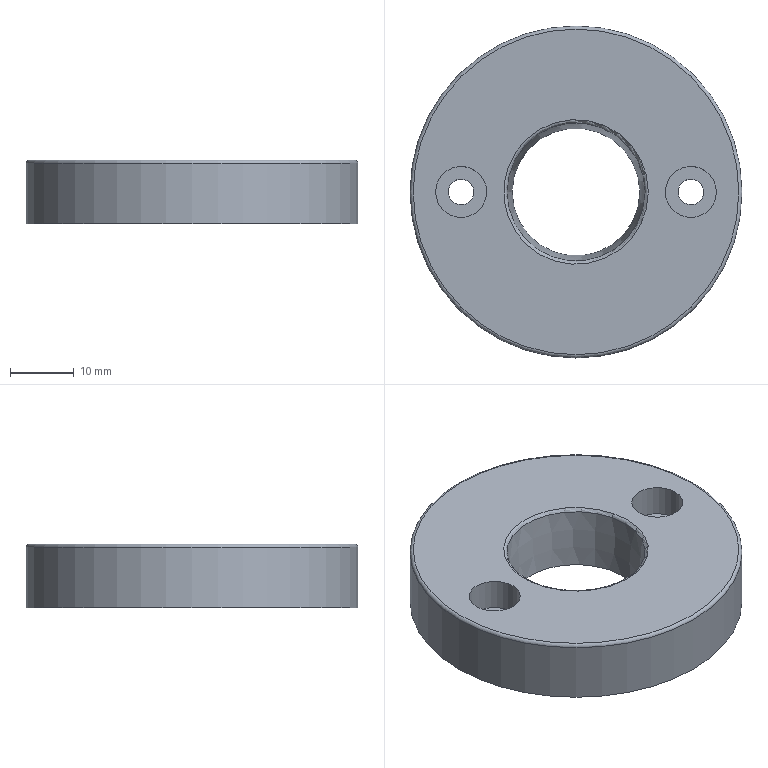Part | STEP file | DISCO_BASE_ALIMENTADOR_PINO | 1 solid | 12 faces | box 52 x 52 x 10 mm | volume 17173 mm3 | cylinder 5 | plane 4 | torus 2 | cone 1 | commonest cylinder face diameters 4 x2 8 x2 52 x1
STEP:
#1=CARTESIAN_POINT('',(0.,0.,0.));
#2=DIRECTION('',(0.,0.,1.));
#3=DIRECTION('',(1.,0.,0.));
#4=AXIS2_PLACEMENT_3D('',#1,#2,#3);
#5=CARTESIAN_POINT('',(-21.51,1.918,5.));
#6=VERTEX_POINT('',#5);
#7=CARTESIAN_POINT('',(-18.,0.,5.));
#8=DIRECTION('',(0.,0.,-1.));
#9=DIRECTION('',(1.,0.,0.));
#10=AXIS2_PLACEMENT_3D('',#7,#8,#9);
#11=CIRCLE('',#10,4.);
#12=CARTESIAN_POINT('',(-16.,0.,5.));
#13=DIRECTION('',(0.,0.,-1.));
#14=DIRECTION('',(-1.,0.,0.));
#15=AXIS2_PLACEMENT_3D('',#12,#13,#14);
#16=PLANE('',#15);
#17=CARTESIAN_POINT('',(2.,0.));
#18=DIRECTION('',(-1.,0.));
#19=AXIS2_PLACEMENT_2D('',#17,#18);
#20=CIRCLE('',#19,4.);
#21=(GEOMETRIC_REPRESENTATION_CONTEXT(2)PARAMETRIC_REPRESENTATION_CONTEXT()REPRESENTATION_CONTEXT('',''));
#22=DEFINITIONAL_REPRESENTATION('',(#20),#21);
#23=PCURVE('',#16,#22);
#24=CARTESIAN_POINT('',(-18.,0.,9.9));
#25=DIRECTION('',(0.,0.,-1.));
#26=DIRECTION('',(0.8776,-0.4794,0.));
#27=AXIS2_PLACEMENT_3D('',#24,#25,#26);
#28=CYLINDRICAL_SURFACE('',#27,4.);
#29=CARTESIAN_POINT('',(-0.5,4.9));
#30=DIRECTION('',(1.,0.));
#31=VECTOR('',#30,1.);
#32=LINE('',#29,#31);
#33=(GEOMETRIC_REPRESENTATION_CONTEXT(2)PARAMETRIC_REPRESENTATION_CONTEXT()REPRESENTATION_CONTEXT('',''));
#34=DEFINITIONAL_REPRESENTATION('',(#32),#33);
#35=PCURVE('',#28,#34);
#36=SURFACE_CURVE('',#11,(#23,#35),.PCURVE_S1.);
#37=EDGE_CURVE('',#6,#6,#36,.T.);
#38=ORIENTED_EDGE('',*,*,#37,.F.);
#39=EDGE_LOOP('',(#38));
#40=FACE_BOUND('',#39,.T.);
#41=CARTESIAN_POINT('',(-16.245,-0.9589,5.));
#42=VERTEX_POINT('',#41);
#43=CARTESIAN_POINT('',(-18.,0.,5.));
#44=DIRECTION('',(0.,0.,-1.));
#45=DIRECTION('',(1.,0.,0.));
#46=AXIS2_PLACEMENT_3D('',#43,#44,#45);
#47=CIRCLE('',#46,2.);
#48=CARTESIAN_POINT('',(2.,0.));
#49=DIRECTION('',(-1.,0.));
#50=AXIS2_PLACEMENT_2D('',#48,#49);
#51=CIRCLE('',#50,2.);
#52=(GEOMETRIC_REPRESENTATION_CONTEXT(2)PARAMETRIC_REPRESENTATION_CONTEXT()REPRESENTATION_CONTEXT('',''));
#53=DEFINITIONAL_REPRESENTATION('',(#51),#52);
#54=PCURVE('',#16,#53);
#55=CARTESIAN_POINT('',(-18.,0.,9.9));
#56=DIRECTION('',(0.,0.,-1.));
#57=DIRECTION('',(0.8776,-0.4794,0.));
#58=AXIS2_PLACEMENT_3D('',#55,#56,#57);
#59=CYLINDRICAL_SURFACE('',#58,2.);
#60=CARTESIAN_POINT('',(-0.5,4.9));
#61=DIRECTION('',(1.,0.));
#62=VECTOR('',#61,1.);
#63=LINE('',#60,#62);
#64=(GEOMETRIC_REPRESENTATION_CONTEXT(2)PARAMETRIC_REPRESENTATION_CONTEXT()REPRESENTATION_CONTEXT('',''));
#65=DEFINITIONAL_REPRESENTATION('',(#63),#64);
#66=PCURVE('',#59,#65);
#67=SURFACE_CURVE('',#47,(#54,#66),.PCURVE_S1.);
#68=EDGE_CURVE('',#42,#42,#67,.T.);
#69=ORIENTED_EDGE('',*,*,#68,.T.);
#70=EDGE_LOOP('',(#69));
#71=FACE_BOUND('',#70,.T.);
#72=ADVANCED_FACE('',(#40,#71),#16,.F.);
#73=CARTESIAN_POINT('',(-16.245,-0.9589,0.));
#74=VERTEX_POINT('',#73);
#75=CARTESIAN_POINT('',(-18.,0.,0.));
#76=DIRECTION('',(0.,0.,-1.));
#77=DIRECTION('',(1.,0.,0.));
#78=AXIS2_PLACEMENT_3D('',#75,#76,#77);
#79=CIRCLE('',#78,2.);
#80=CARTESIAN_POINT('',(-0.5,9.9));
#81=DIRECTION('',(1.,0.));
#82=VECTOR('',#81,1.);
#83=LINE('',#80,#82);
#84=(GEOMETRIC_REPRESENTATION_CONTEXT(2)PARAMETRIC_REPRESENTATION_CONTEXT()REPRESENTATION_CONTEXT('',''));
#85=DEFINITIONAL_REPRESENTATION('',(#83),#84);
#86=PCURVE('',#59,#85);
#87=CARTESIAN_POINT('',(0.,0.,0.));
#88=DIRECTION('',(0.,0.,1.));
#89=DIRECTION('',(1.,0.,0.));
#90=AXIS2_PLACEMENT_3D('',#87,#88,#89);
#91=PLANE('',#90);
#92=CARTESIAN_POINT('',(-16.,0.));
#93=CARTESIAN_POINT('',(-16.,-3.464));
#94=CARTESIAN_POINT('',(-19.,-1.732));
#95=CARTESIAN_POINT('',(-22.,0.));
#96=CARTESIAN_POINT('',(-19.,1.732));
#97=CARTESIAN_POINT('',(-16.,3.464));
#98=CARTESIAN_POINT('',(-16.,0.));
#99=(BOUNDED_CURVE()B_SPLINE_CURVE(2,(#92,#93,#94,#95,#96,#97,#98),.UNSPECIFIED.,.T.,.F.)B_SPLINE_CURVE_WITH_KNOTS((1,2,2,2,2,1),(-2.094,0.,2.094,4.189,6.283,8.378),.UNSPECIFIED.)CURVE()GEOMETRIC_REPRESENTATION_ITEM()RATIONAL_B_SPLINE_CURVE((1.,0.5,1.,0.5,1.,0.5,1.))REPRESENTATION_ITEM(''));
#100=(GEOMETRIC_REPRESENTATION_CONTEXT(2)PARAMETRIC_REPRESENTATION_CONTEXT()REPRESENTATION_CONTEXT('',''));
#101=DEFINITIONAL_REPRESENTATION('',(#99),#100);
#102=PCURVE('',#91,#101);
#103=SURFACE_CURVE('',#79,(#86,#102),.PCURVE_S1.);
#104=EDGE_CURVE('',#74,#74,#103,.T.);
#105=ORIENTED_EDGE('',*,*,#104,.F.);
#106=CARTESIAN_POINT('',(-16.245,-0.9589,5.));
#107=CARTESIAN_POINT('',(-16.245,-0.9589,0.));
#108=B_SPLINE_CURVE_WITH_KNOTS('',1,(#106,#107),.UNSPECIFIED.,.F.,.F.,(2,2),(4.9,9.9),.PIECEWISE_BEZIER_KNOTS.);
#109=CARTESIAN_POINT('',(0.,0.));
#110=DIRECTION('',(0.,1.));
#111=VECTOR('',#110,1.);
#112=LINE('',#109,#111);
#113=(GEOMETRIC_REPRESENTATION_CONTEXT(2)PARAMETRIC_REPRESENTATION_CONTEXT()REPRESENTATION_CONTEXT('',''));
#114=DEFINITIONAL_REPRESENTATION('',(#112),#113);
#115=PCURVE('',#59,#114);
#116=CARTESIAN_POINT('',(6.283,0.));
#117=DIRECTION('',(0.,1.));
#118=VECTOR('',#117,1.);
#119=LINE('',#116,#118);
#120=(GEOMETRIC_REPRESENTATION_CONTEXT(2)PARAMETRIC_REPRESENTATION_CONTEXT()REPRESENTATION_CONTEXT('',''));
#121=DEFINITIONAL_REPRESENTATION('',(#119),#120);
#122=PCURVE('',#59,#121);
#123=SEAM_CURVE('',#108,(#115,#122),.PCURVE_S1.);
#124=EDGE_CURVE('',#42,#74,#123,.T.);
#125=ORIENTED_EDGE('',*,*,#124,.F.);
#126=ORIENTED_EDGE('',*,*,#68,.T.);
#127=ORIENTED_EDGE('',*,*,#124,.T.);
#128=EDGE_LOOP('',(#105,#125,#126,#127));
#129=FACE_BOUND('',#128,.F.);
#130=ADVANCED_FACE('',(#129),#59,.F.);
#131=CARTESIAN_POINT('',(-21.51,1.918,10.));
#132=VERTEX_POINT('',#131);
#133=CARTESIAN_POINT('',(-18.,0.,10.));
#134=DIRECTION('',(0.,0.,-1.));
#135=DIRECTION('',(1.,0.,0.));
#136=AXIS2_PLACEMENT_3D('',#133,#134,#135);
#137=CIRCLE('',#136,4.);
#138=CARTESIAN_POINT('',(-0.5,-0.1));
#139=DIRECTION('',(1.,0.));
#140=VECTOR('',#139,1.);
#141=LINE('',#138,#140);
#142=(GEOMETRIC_REPRESENTATION_CONTEXT(2)PARAMETRIC_REPRESENTATION_CONTEXT()REPRESENTATION_CONTEXT('',''));
#143=DEFINITIONAL_REPRESENTATION('',(#141),#142);
#144=PCURVE('',#28,#143);
#145=CARTESIAN_POINT('',(0.,0.,10.));
#146=DIRECTION('',(0.,0.,1.));
#147=DIRECTION('',(1.,0.,0.));
#148=AXIS2_PLACEMENT_3D('',#145,#146,#147);
#149=PLANE('',#148);
#150=CARTESIAN_POINT('',(-14.,0.));
#151=CARTESIAN_POINT('',(-14.,-6.928));
#152=CARTESIAN_POINT('',(-20.,-3.464));
#153=CARTESIAN_POINT('',(-26.,0.));
#154=CARTESIAN_POINT('',(-20.,3.464));
#155=CARTESIAN_POINT('',(-14.,6.928));
#156=CARTESIAN_POINT('',(-14.,0.));
#157=(BOUNDED_CURVE()B_SPLINE_CURVE(2,(#150,#151,#152,#153,#154,#155,#156),.UNSPECIFIED.,.T.,.F.)B_SPLINE_CURVE_WITH_KNOTS((1,2,2,2,2,1),(-2.094,0.,2.094,4.189,6.283,8.378),.UNSPECIFIED.)CURVE()GEOMETRIC_REPRESENTATION_ITEM()RATIONAL_B_SPLINE_CURVE((1.,0.5,1.,0.5,1.,0.5,1.))REPRESENTATION_ITEM(''));
#158=(GEOMETRIC_REPRESENTATION_CONTEXT(2)PARAMETRIC_REPRESENTATION_CONTEXT()REPRESENTATION_CONTEXT('',''));
#159=DEFINITIONAL_REPRESENTATION('',(#157),#158);
#160=PCURVE('',#149,#159);
#161=SURFACE_CURVE('',#137,(#144,#160),.PCURVE_S1.);
#162=EDGE_CURVE('',#132,#132,#161,.T.);
#163=ORIENTED_EDGE('',*,*,#162,.T.);
#164=CARTESIAN_POINT('',(-21.51,1.918,10.));
#165=CARTESIAN_POINT('',(-21.51,1.918,5.));
#166=B_SPLINE_CURVE_WITH_KNOTS('',1,(#164,#165),.UNSPECIFIED.,.F.,.F.,(2,2),(-0.1,4.9),.PIECEWISE_BEZIER_KNOTS.);
#167=CARTESIAN_POINT('',(9.425,0.));
#168=DIRECTION('',(0.,1.));
#169=VECTOR('',#168,1.);
#170=LINE('',#167,#169);
#171=(GEOMETRIC_REPRESENTATION_CONTEXT(2)PARAMETRIC_REPRESENTATION_CONTEXT()REPRESENTATION_CONTEXT('',''));
#172=DEFINITIONAL_REPRESENTATION('',(#170),#171);
#173=PCURVE('',#28,#172);
#174=CARTESIAN_POINT('',(3.142,0.));
#175=DIRECTION('',(0.,1.));
#176=VECTOR('',#175,1.);
#177=LINE('',#174,#176);
#178=(GEOMETRIC_REPRESENTATION_CONTEXT(2)PARAMETRIC_REPRESENTATION_CONTEXT()REPRESENTATION_CONTEXT('',''));
#179=DEFINITIONAL_REPRESENTATION('',(#177),#178);
#180=PCURVE('',#28,#179);
#181=SEAM_CURVE('',#166,(#173,#180),.PCURVE_S1.);
#182=EDGE_CURVE('',#132,#6,#181,.T.);
#183=ORIENTED_EDGE('',*,*,#182,.T.);
#184=ORIENTED_EDGE('',*,*,#37,.F.);
#185=ORIENTED_EDGE('',*,*,#182,.F.);
#186=EDGE_LOOP('',(#163,#183,#184,#185));
#187=FACE_BOUND('',#186,.F.);
#188=ADVANCED_FACE('',(#187),#28,.F.);
#189=CARTESIAN_POINT('',(-26.,0.,0.));
#190=VERTEX_POINT('',#189);
#191=CARTESIAN_POINT('',(0.,0.,0.));
#192=DIRECTION('',(0.,0.,1.));
#193=DIRECTION('',(1.,0.,0.));
#194=AXIS2_PLACEMENT_3D('',#191,#192,#193);
#195=CIRCLE('',#194,26.);
#196=CARTESIAN_POINT('',(0.,0.));
#197=DIRECTION('',(1.,0.));
#198=AXIS2_PLACEMENT_2D('',#196,#197);
#199=CIRCLE('',#198,26.);
#200=(GEOMETRIC_REPRESENTATION_CONTEXT(2)PARAMETRIC_REPRESENTATION_CONTEXT()REPRESENTATION_CONTEXT('',''));
#201=DEFINITIONAL_REPRESENTATION('',(#199),#200);
#202=PCURVE('',#91,#201);
#203=CARTESIAN_POINT('',(0.,0.,5.));
#204=DIRECTION('',(0.,0.,1.));
#205=DIRECTION('',(1.,0.,0.));
#206=AXIS2_PLACEMENT_3D('',#203,#204,#205);
#207=CYLINDRICAL_SURFACE('',#206,26.);
#208=CARTESIAN_POINT('',(0.,-5.));
#209=DIRECTION('',(1.,0.));
#210=VECTOR('',#209,1.);
#211=LINE('',#208,#210);
#212=(GEOMETRIC_REPRESENTATION_CONTEXT(2)PARAMETRIC_REPRESENTATION_CONTEXT()REPRESENTATION_CONTEXT('',''));
#213=DEFINITIONAL_REPRESENTATION('',(#211),#212);
#214=PCURVE('',#207,#213);
#215=SURFACE_CURVE('',#195,(#202,#214),.PCURVE_S1.);
#216=EDGE_CURVE('',#190,#190,#215,.T.);
#217=ORIENTED_EDGE('',*,*,#216,.F.);
#218=EDGE_LOOP('',(#217));
#219=FACE_BOUND('',#218,.T.);
#220=CARTESIAN_POINT('',(16.245,0.9589,0.));
#221=VERTEX_POINT('',#220);
#222=CARTESIAN_POINT('',(18.,0.,0.));
#223=DIRECTION('',(0.,0.,1.));
#224=DIRECTION('',(1.,0.,0.));
#225=AXIS2_PLACEMENT_3D('',#222,#223,#224);
#226=CIRCLE('',#225,2.);
#227=CARTESIAN_POINT('',(18.,0.));
#228=DIRECTION('',(1.,0.));
#229=AXIS2_PLACEMENT_2D('',#227,#228);
#230=CIRCLE('',#229,2.);
#231=(GEOMETRIC_REPRESENTATION_CONTEXT(2)PARAMETRIC_REPRESENTATION_CONTEXT()REPRESENTATION_CONTEXT('',''));
#232=DEFINITIONAL_REPRESENTATION('',(#230),#231);
#233=PCURVE('',#91,#232);
#234=CARTESIAN_POINT('',(18.,0.,9.9));
#235=DIRECTION('',(0.,0.,-1.));
#236=DIRECTION('',(-0.8776,0.4794,0.));
#237=AXIS2_PLACEMENT_3D('',#234,#235,#236);
#238=CYLINDRICAL_SURFACE('',#237,2.);
#239=CARTESIAN_POINT('',(8.925,9.9));
#240=DIRECTION('',(-1.,0.));
#241=VECTOR('',#240,1.);
#242=LINE('',#239,#241);
#243=(GEOMETRIC_REPRESENTATION_CONTEXT(2)PARAMETRIC_REPRESENTATION_CONTEXT()REPRESENTATION_CONTEXT('',''));
#244=DEFINITIONAL_REPRESENTATION('',(#242),#243);
#245=PCURVE('',#238,#244);
#246=SURFACE_CURVE('',#226,(#233,#245),.PCURVE_S1.);
#247=EDGE_CURVE('',#221,#221,#246,.T.);
#248=ORIENTED_EDGE('',*,*,#247,.T.);
#249=EDGE_LOOP('',(#248));
#250=FACE_BOUND('',#249,.T.);
#251=ORIENTED_EDGE('',*,*,#104,.F.);
#252=EDGE_LOOP('',(#251));
#253=FACE_BOUND('',#252,.T.);
#254=CARTESIAN_POINT('',(-10.,0.,0.));
#255=VERTEX_POINT('',#254);
#256=CARTESIAN_POINT('',(0.,0.,0.));
#257=DIRECTION('',(0.,0.,1.));
#258=DIRECTION('',(1.,0.,0.));
#259=AXIS2_PLACEMENT_3D('',#256,#257,#258);
#260=CIRCLE('',#259,10.);
#261=CARTESIAN_POINT('',(0.,0.));
#262=DIRECTION('',(1.,0.));
#263=AXIS2_PLACEMENT_2D('',#261,#262);
#264=CIRCLE('',#263,10.);
#265=(GEOMETRIC_REPRESENTATION_CONTEXT(2)PARAMETRIC_REPRESENTATION_CONTEXT()REPRESENTATION_CONTEXT('',''));
#266=DEFINITIONAL_REPRESENTATION('',(#264),#265);
#267=PCURVE('',#91,#266);
#268=CARTESIAN_POINT('',(0.,0.,0.));
#269=DIRECTION('',(0.,0.,1.));
#270=DIRECTION('',(-1.,0.,0.));
#271=AXIS2_PLACEMENT_3D('',#268,#269,#270);
#272=CONICAL_SURFACE('',#271,10.,0.08727);
#273=CARTESIAN_POINT('',(-3.142,0.));
#274=DIRECTION('',(1.,0.));
#275=VECTOR('',#274,1.);
#276=LINE('',#273,#275);
#277=(GEOMETRIC_REPRESENTATION_CONTEXT(2)PARAMETRIC_REPRESENTATION_CONTEXT()REPRESENTATION_CONTEXT('',''));
#278=DEFINITIONAL_REPRESENTATION('',(#276),#277);
#279=PCURVE('',#272,#278);
#280=SURFACE_CURVE('',#260,(#267,#279),.PCURVE_S1.);
#281=EDGE_CURVE('',#255,#255,#280,.T.);
#282=ORIENTED_EDGE('',*,*,#281,.T.);
#283=EDGE_LOOP('',(#282));
#284=FACE_BOUND('',#283,.T.);
#285=ADVANCED_FACE('',(#219,#250,#253,#284),#91,.F.);
#286=CARTESIAN_POINT('',(14.49,1.918,5.));
#287=VERTEX_POINT('',#286);
#288=CARTESIAN_POINT('',(18.,0.,5.));
#289=DIRECTION('',(0.,0.,-1.));
#290=DIRECTION('',(1.,0.,0.));
#291=AXIS2_PLACEMENT_3D('',#288,#289,#290);
#292=CIRCLE('',#291,4.);
#293=CARTESIAN_POINT('',(-16.,0.,5.));
#294=DIRECTION('',(0.,0.,-1.));
#295=DIRECTION('',(-1.,0.,0.));
#296=AXIS2_PLACEMENT_3D('',#293,#294,#295);
#297=PLANE('',#296);
#298=CARTESIAN_POINT('',(-34.,0.));
#299=DIRECTION('',(-1.,0.));
#300=AXIS2_PLACEMENT_2D('',#298,#299);
#301=CIRCLE('',#300,4.);
#302=(GEOMETRIC_REPRESENTATION_CONTEXT(2)PARAMETRIC_REPRESENTATION_CONTEXT()REPRESENTATION_CONTEXT('',''));
#303=DEFINITIONAL_REPRESENTATION('',(#301),#302);
#304=PCURVE('',#297,#303);
#305=CARTESIAN_POINT('',(18.,0.,9.9));
#306=DIRECTION('',(0.,0.,-1.));
#307=DIRECTION('',(-0.8776,0.4794,0.));
#308=AXIS2_PLACEMENT_3D('',#305,#306,#307);
#309=CYLINDRICAL_SURFACE('',#308,4.);
#310=CARTESIAN_POINT('',(-3.642,4.9));
#311=DIRECTION('',(1.,0.));
#312=VECTOR('',#311,1.);
#313=LINE('',#310,#312);
#314=(GEOMETRIC_REPRESENTATION_CONTEXT(2)PARAMETRIC_REPRESENTATION_CONTEXT()REPRESENTATION_CONTEXT('',''));
#315=DEFINITIONAL_REPRESENTATION('',(#313),#314);
#316=PCURVE('',#309,#315);
#317=SURFACE_CURVE('',#292,(#304,#316),.PCURVE_S1.);
#318=EDGE_CURVE('',#287,#287,#317,.T.);
#319=ORIENTED_EDGE('',*,*,#318,.F.);
#320=EDGE_LOOP('',(#319));
#321=FACE_BOUND('',#320,.T.);
#322=CARTESIAN_POINT('',(16.245,0.9589,5.));
#323=VERTEX_POINT('',#322);
#324=CARTESIAN_POINT('',(18.,0.,5.));
#325=DIRECTION('',(0.,0.,-1.));
#326=DIRECTION('',(1.,0.,0.));
#327=AXIS2_PLACEMENT_3D('',#324,#325,#326);
#328=CIRCLE('',#327,2.);
#329=CARTESIAN_POINT('',(-34.,0.));
#330=DIRECTION('',(-1.,0.));
#331=AXIS2_PLACEMENT_2D('',#329,#330);
#332=CIRCLE('',#331,2.);
#333=(GEOMETRIC_REPRESENTATION_CONTEXT(2)PARAMETRIC_REPRESENTATION_CONTEXT()REPRESENTATION_CONTEXT('',''));
#334=DEFINITIONAL_REPRESENTATION('',(#332),#333);
#335=PCURVE('',#297,#334);
#336=CARTESIAN_POINT('',(-3.642,4.9));
#337=DIRECTION('',(1.,0.));
#338=VECTOR('',#337,1.);
#339=LINE('',#336,#338);
#340=(GEOMETRIC_REPRESENTATION_CONTEXT(2)PARAMETRIC_REPRESENTATION_CONTEXT()REPRESENTATION_CONTEXT('',''));
#341=DEFINITIONAL_REPRESENTATION('',(#339),#340);
#342=PCURVE('',#238,#341);
#343=SURFACE_CURVE('',#328,(#335,#342),.PCURVE_S1.);
#344=EDGE_CURVE('',#323,#323,#343,.T.);
#345=ORIENTED_EDGE('',*,*,#344,.T.);
#346=EDGE_LOOP('',(#345));
#347=FACE_BOUND('',#346,.T.);
#348=ADVANCED_FACE('',(#321,#347),#297,.F.);
#349=CARTESIAN_POINT('',(14.49,1.918,10.));
#350=VERTEX_POINT('',#349);
#351=CARTESIAN_POINT('',(18.,0.,10.));
#352=DIRECTION('',(0.,0.,-1.));
#353=DIRECTION('',(1.,0.,0.));
#354=AXIS2_PLACEMENT_3D('',#351,#352,#353);
#355=CIRCLE('',#354,4.);
#356=CARTESIAN_POINT('',(-3.642,-0.1));
#357=DIRECTION('',(1.,0.));
#358=VECTOR('',#357,1.);
#359=LINE('',#356,#358);
#360=(GEOMETRIC_REPRESENTATION_CONTEXT(2)PARAMETRIC_REPRESENTATION_CONTEXT()REPRESENTATION_CONTEXT('',''));
#361=DEFINITIONAL_REPRESENTATION('',(#359),#360);
#362=PCURVE('',#309,#361);
#363=CARTESIAN_POINT('',(22.,0.));
#364=CARTESIAN_POINT('',(22.,-6.928));
#365=CARTESIAN_POINT('',(16.,-3.464));
#366=CARTESIAN_POINT('',(10.,0.));
#367=CARTESIAN_POINT('',(16.,3.464));
#368=CARTESIAN_POINT('',(22.,6.928));
#369=CARTESIAN_POINT('',(22.,0.));
#370=(BOUNDED_CURVE()B_SPLINE_CURVE(2,(#363,#364,#365,#366,#367,#368,#369),.UNSPECIFIED.,.T.,.F.)B_SPLINE_CURVE_WITH_KNOTS((1,2,2,2,2,1),(-2.094,0.,2.094,4.189,6.283,8.378),.UNSPECIFIED.)CURVE()GEOMETRIC_REPRESENTATION_ITEM()RATIONAL_B_SPLINE_CURVE((1.,0.5,1.,0.5,1.,0.5,1.))REPRESENTATION_ITEM(''));
#371=(GEOMETRIC_REPRESENTATION_CONTEXT(2)PARAMETRIC_REPRESENTATION_CONTEXT()REPRESENTATION_CONTEXT('',''));
#372=DEFINITIONAL_REPRESENTATION('',(#370),#371);
#373=PCURVE('',#149,#372);
#374=SURFACE_CURVE('',#355,(#362,#373),.PCURVE_S1.);
#375=EDGE_CURVE('',#350,#350,#374,.T.);
#376=ORIENTED_EDGE('',*,*,#375,.T.);
#377=CARTESIAN_POINT('',(14.49,1.918,10.));
#378=CARTESIAN_POINT('',(14.49,1.918,5.));
#379=B_SPLINE_CURVE_WITH_KNOTS('',1,(#377,#378),.UNSPECIFIED.,.F.,.F.,(2,2),(-0.1,4.9),.PIECEWISE_BEZIER_KNOTS.);
#380=CARTESIAN_POINT('',(6.283,0.));
#381=DIRECTION('',(0.,1.));
#382=VECTOR('',#381,1.);
#383=LINE('',#380,#382);
#384=(GEOMETRIC_REPRESENTATION_CONTEXT(2)PARAMETRIC_REPRESENTATION_CONTEXT()REPRESENTATION_CONTEXT('',''));
#385=DEFINITIONAL_REPRESENTATION('',(#383),#384);
#386=PCURVE('',#309,#385);
#387=CARTESIAN_POINT('',(0.,0.));
#388=DIRECTION('',(0.,1.));
#389=VECTOR('',#388,1.);
#390=LINE('',#387,#389);
#391=(GEOMETRIC_REPRESENTATION_CONTEXT(2)PARAMETRIC_REPRESENTATION_CONTEXT()REPRESENTATION_CONTEXT('',''));
#392=DEFINITIONAL_REPRESENTATION('',(#390),#391);
#393=PCURVE('',#309,#392);
#394=SEAM_CURVE('',#379,(#386,#393),.PCURVE_S1.);
#395=EDGE_CURVE('',#350,#287,#394,.T.);
#396=ORIENTED_EDGE('',*,*,#395,.T.);
#397=ORIENTED_EDGE('',*,*,#318,.F.);
#398=ORIENTED_EDGE('',*,*,#395,.F.);
#399=EDGE_LOOP('',(#376,#396,#397,#398));
#400=FACE_BOUND('',#399,.F.);
#401=ADVANCED_FACE('',(#400),#309,.F.);
#402=ORIENTED_EDGE('',*,*,#247,.T.);
#403=CARTESIAN_POINT('',(16.245,0.9589,5.));
#404=CARTESIAN_POINT('',(16.245,0.9589,0.));
#405=B_SPLINE_CURVE_WITH_KNOTS('',1,(#403,#404),.UNSPECIFIED.,.F.,.F.,(2,2),(4.9,9.9),.PIECEWISE_BEZIER_KNOTS.);
#406=CARTESIAN_POINT('',(0.,0.));
#407=DIRECTION('',(0.,1.));
#408=VECTOR('',#407,1.);
#409=LINE('',#406,#408);
#410=(GEOMETRIC_REPRESENTATION_CONTEXT(2)PARAMETRIC_REPRESENTATION_CONTEXT()REPRESENTATION_CONTEXT('',''));
#411=DEFINITIONAL_REPRESENTATION('',(#409),#410);
#412=PCURVE('',#238,#411);
#413=CARTESIAN_POINT('',(6.283,0.));
#414=DIRECTION('',(0.,1.));
#415=VECTOR('',#414,1.);
#416=LINE('',#413,#415);
#417=(GEOMETRIC_REPRESENTATION_CONTEXT(2)PARAMETRIC_REPRESENTATION_CONTEXT()REPRESENTATION_CONTEXT('',''));
#418=DEFINITIONAL_REPRESENTATION('',(#416),#417);
#419=PCURVE('',#238,#418);
#420=SEAM_CURVE('',#405,(#412,#419),.PCURVE_S1.);
#421=EDGE_CURVE('',#323,#221,#420,.T.);
#422=ORIENTED_EDGE('',*,*,#421,.F.);
#423=ORIENTED_EDGE('',*,*,#344,.T.);
#424=ORIENTED_EDGE('',*,*,#421,.T.);
#425=EDGE_LOOP('',(#402,#422,#423,#424));
#426=FACE_BOUND('',#425,.F.);
#427=ADVANCED_FACE('',(#426),#238,.F.);
#428=CARTESIAN_POINT('',(-26.,0.,9.5));
#429=VERTEX_POINT('',#428);
#430=CARTESIAN_POINT('',(26.,0.,9.5));
#431=VERTEX_POINT('',#430);
#432=CARTESIAN_POINT('',(0.,0.,9.5));
#433=DIRECTION('',(0.,0.,1.));
#434=DIRECTION('',(1.,0.,0.));
#435=AXIS2_PLACEMENT_3D('',#432,#433,#434);
#436=CIRCLE('',#435,26.);
#437=CARTESIAN_POINT('',(0.,4.5));
#438=DIRECTION('',(1.,0.));
#439=VECTOR('',#438,1.);
#440=LINE('',#437,#439);
#441=(GEOMETRIC_REPRESENTATION_CONTEXT(2)PARAMETRIC_REPRESENTATION_CONTEXT()REPRESENTATION_CONTEXT('',''));
#442=DEFINITIONAL_REPRESENTATION('',(#440),#441);
#443=PCURVE('',#207,#442);
#444=CARTESIAN_POINT('',(0.,0.,9.5));
#445=DIRECTION('',(0.,0.,1.));
#446=DIRECTION('',(1.,0.,0.));
#447=AXIS2_PLACEMENT_3D('',#444,#445,#446);
#448=TOROIDAL_SURFACE('',#447,25.5,0.5);
#449=CARTESIAN_POINT('',(0.,6.283));
#450=DIRECTION('',(1.,0.));
#451=VECTOR('',#450,1.);
#452=LINE('',#449,#451);
#453=(GEOMETRIC_REPRESENTATION_CONTEXT(2)PARAMETRIC_REPRESENTATION_CONTEXT()REPRESENTATION_CONTEXT('',''));
#454=DEFINITIONAL_REPRESENTATION('',(#452),#453);
#455=PCURVE('',#448,#454);
#456=SURFACE_CURVE('',#436,(#443,#455),.PCURVE_S1.);
#457=EDGE_CURVE('',#429,#431,#456,.T.);
#458=ORIENTED_EDGE('',*,*,#457,.F.);
#459=CARTESIAN_POINT('',(-26.,0.,0.));
#460=CARTESIAN_POINT('',(-26.,0.,9.5));
#461=B_SPLINE_CURVE_WITH_KNOTS('',1,(#459,#460),.UNSPECIFIED.,.F.,.F.,(2,2),(-5.,4.5),.PIECEWISE_BEZIER_KNOTS.);
#462=CARTESIAN_POINT('',(3.142,0.));
#463=DIRECTION('',(0.,1.));
#464=VECTOR('',#463,1.);
#465=LINE('',#462,#464);
#466=(GEOMETRIC_REPRESENTATION_CONTEXT(2)PARAMETRIC_REPRESENTATION_CONTEXT()REPRESENTATION_CONTEXT('',''));
#467=DEFINITIONAL_REPRESENTATION('',(#465),#466);
#468=PCURVE('',#207,#467);
#469=CARTESIAN_POINT('',(9.425,0.));
#470=DIRECTION('',(0.,1.));
#471=VECTOR('',#470,1.);
#472=LINE('',#469,#471);
#473=(GEOMETRIC_REPRESENTATION_CONTEXT(2)PARAMETRIC_REPRESENTATION_CONTEXT()REPRESENTATION_CONTEXT('',''));
#474=DEFINITIONAL_REPRESENTATION('',(#472),#473);
#475=PCURVE('',#207,#474);
#476=SEAM_CURVE('',#461,(#468,#475),.PCURVE_S1.);
#477=EDGE_CURVE('',#190,#429,#476,.T.);
#478=ORIENTED_EDGE('',*,*,#477,.F.);
#479=ORIENTED_EDGE('',*,*,#216,.T.);
#480=ORIENTED_EDGE('',*,*,#477,.T.);
#481=CARTESIAN_POINT('',(0.,0.,9.5));
#482=DIRECTION('',(0.,0.,1.));
#483=DIRECTION('',(1.,0.,0.));
#484=AXIS2_PLACEMENT_3D('',#481,#482,#483);
#485=CIRCLE('',#484,26.);
#486=CARTESIAN_POINT('',(0.,4.5));
#487=DIRECTION('',(1.,0.));
#488=VECTOR('',#487,1.);
#489=LINE('',#486,#488);
#490=(GEOMETRIC_REPRESENTATION_CONTEXT(2)PARAMETRIC_REPRESENTATION_CONTEXT()REPRESENTATION_CONTEXT('',''));
#491=DEFINITIONAL_REPRESENTATION('',(#489),#490);
#492=PCURVE('',#207,#491);
#493=CARTESIAN_POINT('',(-6.283,6.283));
#494=DIRECTION('',(1.,0.));
#495=VECTOR('',#494,1.);
#496=LINE('',#493,#495);
#497=(GEOMETRIC_REPRESENTATION_CONTEXT(2)PARAMETRIC_REPRESENTATION_CONTEXT()REPRESENTATION_CONTEXT('',''));
#498=DEFINITIONAL_REPRESENTATION('',(#496),#497);
#499=PCURVE('',#448,#498);
#500=SURFACE_CURVE('',#485,(#492,#499),.PCURVE_S1.);
#501=EDGE_CURVE('',#431,#429,#500,.T.);
#502=ORIENTED_EDGE('',*,*,#501,.F.);
#503=EDGE_LOOP('',(#458,#478,#479,#480,#502));
#504=FACE_BOUND('',#503,.T.);
#505=ADVANCED_FACE('',(#504),#207,.T.);
#506=CARTESIAN_POINT('',(25.5,0.,10.));
#507=VERTEX_POINT('',#506);
#508=CARTESIAN_POINT('',(0.,0.,10.));
#509=DIRECTION('',(0.,0.,1.));
#510=DIRECTION('',(1.,0.,0.));
#511=AXIS2_PLACEMENT_3D('',#508,#509,#510);
#512=CIRCLE('',#511,25.5);
#513=CARTESIAN_POINT('',(0.,7.854));
#514=DIRECTION('',(1.,0.));
#515=VECTOR('',#514,1.);
#516=LINE('',#513,#515);
#517=(GEOMETRIC_REPRESENTATION_CONTEXT(2)PARAMETRIC_REPRESENTATION_CONTEXT()REPRESENTATION_CONTEXT('',''));
#518=DEFINITIONAL_REPRESENTATION('',(#516),#517);
#519=PCURVE('',#448,#518);
#520=CARTESIAN_POINT('',(0.,0.));
#521=DIRECTION('',(1.,0.));
#522=AXIS2_PLACEMENT_2D('',#520,#521);
#523=CIRCLE('',#522,25.5);
#524=(GEOMETRIC_REPRESENTATION_CONTEXT(2)PARAMETRIC_REPRESENTATION_CONTEXT()REPRESENTATION_CONTEXT('',''));
#525=DEFINITIONAL_REPRESENTATION('',(#523),#524);
#526=PCURVE('',#149,#525);
#527=SURFACE_CURVE('',#512,(#519,#526),.PCURVE_S1.);
#528=EDGE_CURVE('',#507,#507,#527,.T.);
#529=ORIENTED_EDGE('',*,*,#528,.F.);
#530=CARTESIAN_POINT('',(26.,0.,9.5));
#531=CARTESIAN_POINT('',(26.,0.,9.634));
#532=CARTESIAN_POINT('',(25.957,0.,9.764));
#533=CARTESIAN_POINT('',(25.876,0.,9.876));
#534=CARTESIAN_POINT('',(25.764,0.,9.957));
#535=CARTESIAN_POINT('',(25.634,0.,10.));
#536=CARTESIAN_POINT('',(25.5,0.,10.));
#537=(BOUNDED_CURVE()B_SPLINE_CURVE(6,(#530,#531,#532,#533,#534,#535,#536),.UNSPECIFIED.,.F.,.F.)B_SPLINE_CURVE_WITH_KNOTS((7,7),(0.,1.571),.PIECEWISE_BEZIER_KNOTS.)CURVE()GEOMETRIC_REPRESENTATION_ITEM()RATIONAL_B_SPLINE_CURVE((1.031,1.01,0.9979,0.994,0.9979,1.01,1.031))REPRESENTATION_ITEM(''));
#538=CARTESIAN_POINT('',(0.,6.283));
#539=DIRECTION('',(0.,1.));
#540=VECTOR('',#539,1.);
#541=LINE('',#538,#540);
#542=(GEOMETRIC_REPRESENTATION_CONTEXT(2)PARAMETRIC_REPRESENTATION_CONTEXT()REPRESENTATION_CONTEXT('',''));
#543=DEFINITIONAL_REPRESENTATION('',(#541),#542);
#544=PCURVE('',#448,#543);
#545=CARTESIAN_POINT('',(6.283,6.283));
#546=DIRECTION('',(0.,1.));
#547=VECTOR('',#546,1.);
#548=LINE('',#545,#547);
#549=(GEOMETRIC_REPRESENTATION_CONTEXT(2)PARAMETRIC_REPRESENTATION_CONTEXT()REPRESENTATION_CONTEXT('',''));
#550=DEFINITIONAL_REPRESENTATION('',(#548),#549);
#551=PCURVE('',#448,#550);
#552=SEAM_CURVE('',#537,(#544,#551),.PCURVE_S1.);
#553=EDGE_CURVE('',#431,#507,#552,.T.);
#554=ORIENTED_EDGE('',*,*,#553,.F.);
#555=ORIENTED_EDGE('',*,*,#501,.T.);
#556=ORIENTED_EDGE('',*,*,#457,.T.);
#557=ORIENTED_EDGE('',*,*,#553,.T.);
#558=EDGE_LOOP('',(#529,#554,#555,#556,#557));
#559=FACE_BOUND('',#558,.T.);
#560=ADVANCED_FACE('',(#559),#448,.T.);
#561=CARTESIAN_POINT('',(-10.835,0.,9.544));
#562=VERTEX_POINT('',#561);
#563=CARTESIAN_POINT('',(10.835,0.000000191,9.544));
#564=VERTEX_POINT('',#563);
#565=CARTESIAN_POINT('',(0.,0.,9.544));
#566=DIRECTION('',(0.,0.,1.));
#567=DIRECTION('',(1.,0.,0.));
#568=AXIS2_PLACEMENT_3D('',#565,#566,#567);
#569=CIRCLE('',#568,10.835);
#570=CARTESIAN_POINT('',(-3.142,9.544));
#571=DIRECTION('',(1.,0.));
#572=VECTOR('',#571,1.);
#573=LINE('',#570,#572);
#574=(GEOMETRIC_REPRESENTATION_CONTEXT(2)PARAMETRIC_REPRESENTATION_CONTEXT()REPRESENTATION_CONTEXT('',''));
#575=DEFINITIONAL_REPRESENTATION('',(#573),#574);
#576=PCURVE('',#272,#575);
#577=CARTESIAN_POINT('',(0.,0.,9.5));
#578=DIRECTION('',(0.,0.,1.));
#579=DIRECTION('',(1.,0.,0.));
#580=AXIS2_PLACEMENT_3D('',#577,#578,#579);
#581=TOROIDAL_SURFACE('',#580,11.333,0.5);
#582=CARTESIAN_POINT('',(0.,9.338));
#583=DIRECTION('',(1.,0.));
#584=VECTOR('',#583,1.);
#585=LINE('',#582,#584);
#586=(GEOMETRIC_REPRESENTATION_CONTEXT(2)PARAMETRIC_REPRESENTATION_CONTEXT()REPRESENTATION_CONTEXT('',''));
#587=DEFINITIONAL_REPRESENTATION('',(#585),#586);
#588=PCURVE('',#581,#587);
#589=SURFACE_CURVE('',#569,(#576,#588),.PCURVE_S1.);
#590=EDGE_CURVE('',#562,#564,#589,.T.);
#591=ORIENTED_EDGE('',*,*,#590,.F.);
#592=CARTESIAN_POINT('',(-10.,0.,0.));
#593=CARTESIAN_POINT('',(-10.835,0.,9.544));
#594=B_SPLINE_CURVE_WITH_KNOTS('',1,(#592,#593),.UNSPECIFIED.,.F.,.F.,(2,2),(0.,9.58),.PIECEWISE_BEZIER_KNOTS.);
#595=CARTESIAN_POINT('',(0.,0.));
#596=DIRECTION('',(0.,1.));
#597=VECTOR('',#596,1.);
#598=LINE('',#595,#597);
#599=(GEOMETRIC_REPRESENTATION_CONTEXT(2)PARAMETRIC_REPRESENTATION_CONTEXT()REPRESENTATION_CONTEXT('',''));
#600=DEFINITIONAL_REPRESENTATION('',(#598),#599);
#601=PCURVE('',#272,#600);
#602=CARTESIAN_POINT('',(6.283,0.));
#603=DIRECTION('',(0.,1.));
#604=VECTOR('',#603,1.);
#605=LINE('',#602,#604);
#606=(GEOMETRIC_REPRESENTATION_CONTEXT(2)PARAMETRIC_REPRESENTATION_CONTEXT()REPRESENTATION_CONTEXT('',''));
#607=DEFINITIONAL_REPRESENTATION('',(#605),#606);
#608=PCURVE('',#272,#607);
#609=SEAM_CURVE('',#594,(#601,#608),.PCURVE_S1.);
#610=EDGE_CURVE('',#255,#562,#609,.T.);
#611=ORIENTED_EDGE('',*,*,#610,.F.);
#612=ORIENTED_EDGE('',*,*,#281,.T.);
#613=ORIENTED_EDGE('',*,*,#610,.T.);
#614=CARTESIAN_POINT('',(0.,0.,9.544));
#615=DIRECTION('',(0.,0.,1.));
#616=DIRECTION('',(1.,0.,0.));
#617=AXIS2_PLACEMENT_3D('',#614,#615,#616);
#618=CIRCLE('',#617,10.835);
#619=CARTESIAN_POINT('',(3.142,9.544));
#620=DIRECTION('',(1.,0.));
#621=VECTOR('',#620,1.);
#622=LINE('',#619,#621);
#623=(GEOMETRIC_REPRESENTATION_CONTEXT(2)PARAMETRIC_REPRESENTATION_CONTEXT()REPRESENTATION_CONTEXT('',''));
#624=DEFINITIONAL_REPRESENTATION('',(#622),#623);
#625=PCURVE('',#272,#624);
#626=CARTESIAN_POINT('',(0.,9.338));
#627=DIRECTION('',(1.,0.));
#628=VECTOR('',#627,1.);
#629=LINE('',#626,#628);
#630=(GEOMETRIC_REPRESENTATION_CONTEXT(2)PARAMETRIC_REPRESENTATION_CONTEXT()REPRESENTATION_CONTEXT('',''));
#631=DEFINITIONAL_REPRESENTATION('',(#629),#630);
#632=PCURVE('',#581,#631);
#633=SURFACE_CURVE('',#618,(#625,#632),.PCURVE_S1.);
#634=EDGE_CURVE('',#564,#562,#633,.T.);
#635=ORIENTED_EDGE('',*,*,#634,.F.);
#636=EDGE_LOOP('',(#591,#611,#612,#613,#635));
#637=FACE_BOUND('',#636,.F.);
#638=ADVANCED_FACE('',(#637),#272,.F.);
#639=ORIENTED_EDGE('',*,*,#528,.T.);
#640=EDGE_LOOP('',(#639));
#641=FACE_BOUND('',#640,.T.);
#642=CARTESIAN_POINT('',(11.333,0.0000002,10.));
#643=VERTEX_POINT('',#642);
#644=CARTESIAN_POINT('',(0.,0.,10.));
#645=DIRECTION('',(0.,0.,1.));
#646=DIRECTION('',(1.,0.,0.));
#647=AXIS2_PLACEMENT_3D('',#644,#645,#646);
#648=CIRCLE('',#647,11.333);
#649=CARTESIAN_POINT('',(0.,0.));
#650=DIRECTION('',(1.,0.));
#651=AXIS2_PLACEMENT_2D('',#649,#650);
#652=CIRCLE('',#651,11.333);
#653=(GEOMETRIC_REPRESENTATION_CONTEXT(2)PARAMETRIC_REPRESENTATION_CONTEXT()REPRESENTATION_CONTEXT('',''));
#654=DEFINITIONAL_REPRESENTATION('',(#652),#653);
#655=PCURVE('',#149,#654);
#656=CARTESIAN_POINT('',(0.,7.854));
#657=DIRECTION('',(1.,0.));
#658=VECTOR('',#657,1.);
#659=LINE('',#656,#658);
#660=(GEOMETRIC_REPRESENTATION_CONTEXT(2)PARAMETRIC_REPRESENTATION_CONTEXT()REPRESENTATION_CONTEXT('',''));
#661=DEFINITIONAL_REPRESENTATION('',(#659),#660);
#662=PCURVE('',#581,#661);
#663=SURFACE_CURVE('',#648,(#655,#662),.PCURVE_S1.);
#664=EDGE_CURVE('',#643,#643,#663,.T.);
#665=ORIENTED_EDGE('',*,*,#664,.F.);
#666=EDGE_LOOP('',(#665));
#667=FACE_BOUND('',#666,.T.);
#668=ORIENTED_EDGE('',*,*,#375,.T.);
#669=EDGE_LOOP('',(#668));
#670=FACE_BOUND('',#669,.T.);
#671=ORIENTED_EDGE('',*,*,#162,.T.);
#672=EDGE_LOOP('',(#671));
#673=FACE_BOUND('',#672,.T.);
#674=ADVANCED_FACE('',(#641,#667,#670,#673),#149,.T.);
#675=ORIENTED_EDGE('',*,*,#664,.T.);
#676=CARTESIAN_POINT('',(11.333,0.0000002,10.));
#677=CARTESIAN_POINT('',(11.207,0.000000198,10.));
#678=CARTESIAN_POINT('',(11.084,0.000000195,9.962));
#679=CARTESIAN_POINT('',(10.976,0.000000194,9.889));
#680=CARTESIAN_POINT('',(10.894,0.000000192,9.788));
#681=CARTESIAN_POINT('',(10.846,0.000000191,9.669));
#682=CARTESIAN_POINT('',(10.835,0.000000191,9.544));
#683=(BOUNDED_CURVE()B_SPLINE_CURVE(6,(#676,#677,#678,#679,#680,#681,#682),.UNSPECIFIED.,.F.,.F.)B_SPLINE_CURVE_WITH_KNOTS((7,7),(1.571,3.054),.PIECEWISE_BEZIER_KNOTS.)CURVE()GEOMETRIC_REPRESENTATION_ITEM()RATIONAL_B_SPLINE_CURVE((1.028,1.009,0.9981,0.9946,0.9981,1.009,1.028))REPRESENTATION_ITEM(''));
#684=CARTESIAN_POINT('',(6.283,6.283));
#685=DIRECTION('',(0.,1.));
#686=VECTOR('',#685,1.);
#687=LINE('',#684,#686);
#688=(GEOMETRIC_REPRESENTATION_CONTEXT(2)PARAMETRIC_REPRESENTATION_CONTEXT()REPRESENTATION_CONTEXT('',''));
#689=DEFINITIONAL_REPRESENTATION('',(#687),#688);
#690=PCURVE('',#581,#689);
#691=CARTESIAN_POINT('',(0.000000018,6.283));
#692=DIRECTION('',(0.,1.));
#693=VECTOR('',#692,1.);
#694=LINE('',#691,#693);
#695=(GEOMETRIC_REPRESENTATION_CONTEXT(2)PARAMETRIC_REPRESENTATION_CONTEXT()REPRESENTATION_CONTEXT('',''));
#696=DEFINITIONAL_REPRESENTATION('',(#694),#695);
#697=PCURVE('',#581,#696);
#698=SEAM_CURVE('',#683,(#690,#697),.PCURVE_S1.);
#699=EDGE_CURVE('',#643,#564,#698,.T.);
#700=ORIENTED_EDGE('',*,*,#699,.T.);
#701=ORIENTED_EDGE('',*,*,#590,.F.);
#702=ORIENTED_EDGE('',*,*,#634,.F.);
#703=ORIENTED_EDGE('',*,*,#699,.F.);
#704=EDGE_LOOP('',(#675,#700,#701,#702,#703));
#705=FACE_BOUND('',#704,.T.);
#706=ADVANCED_FACE('',(#705),#581,.T.);
#707=CLOSED_SHELL('',(#72,#130,#188,#285,#348,#401,#427,#505,#560,#638,#674,#706));
#708=MANIFOLD_SOLID_BREP('',#707);
#709=(LENGTH_UNIT()NAMED_UNIT(*)SI_UNIT(.MILLI.,.METRE.));
#710=UNCERTAINTY_MEASURE_WITH_UNIT(LENGTH_MEASURE(0.00001),#709,'','');
#711=(NAMED_UNIT(*)PLANE_ANGLE_UNIT()SI_UNIT($,.RADIAN.));
#712=(NAMED_UNIT(*)SI_UNIT($,.STERADIAN.)SOLID_ANGLE_UNIT());
#713=(GEOMETRIC_REPRESENTATION_CONTEXT(3)GLOBAL_UNCERTAINTY_ASSIGNED_CONTEXT((#710))GLOBAL_UNIT_ASSIGNED_CONTEXT((#709,#711,#712))REPRESENTATION_CONTEXT('',''));
#714=ADVANCED_BREP_SHAPE_REPRESENTATION('',(#4,#708),#713);